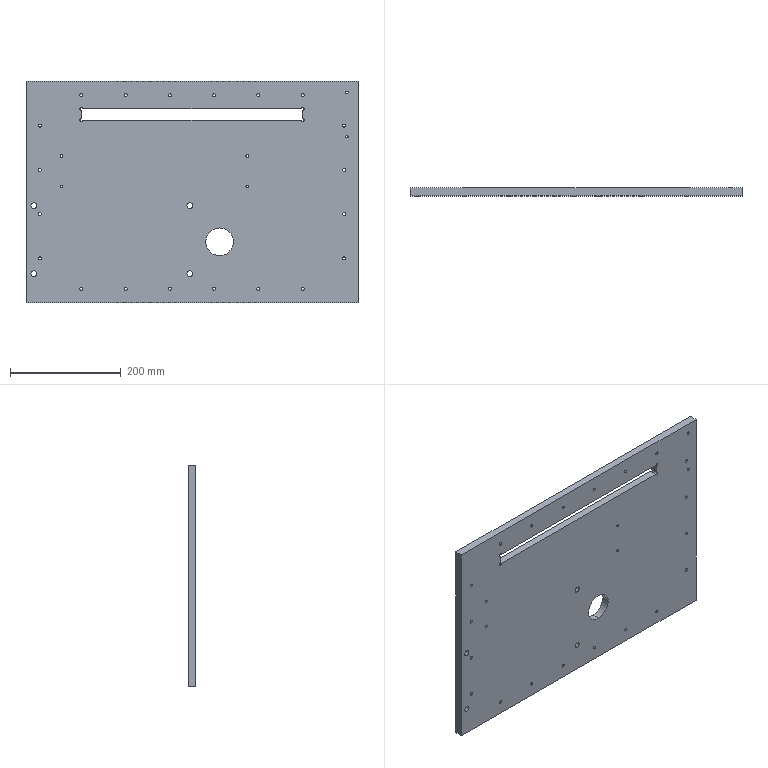Part | STEP file | PN_0071 table plate | 1 solid | 138 faces | box 600 x 14 x 400 mm | volume 3201054 mm3 | cylinder 108 | plane 30 | commonest cylinder face diameters 5.5 x40 10 x40 5 x14 10.2 x8 4.2 x4 50 x2